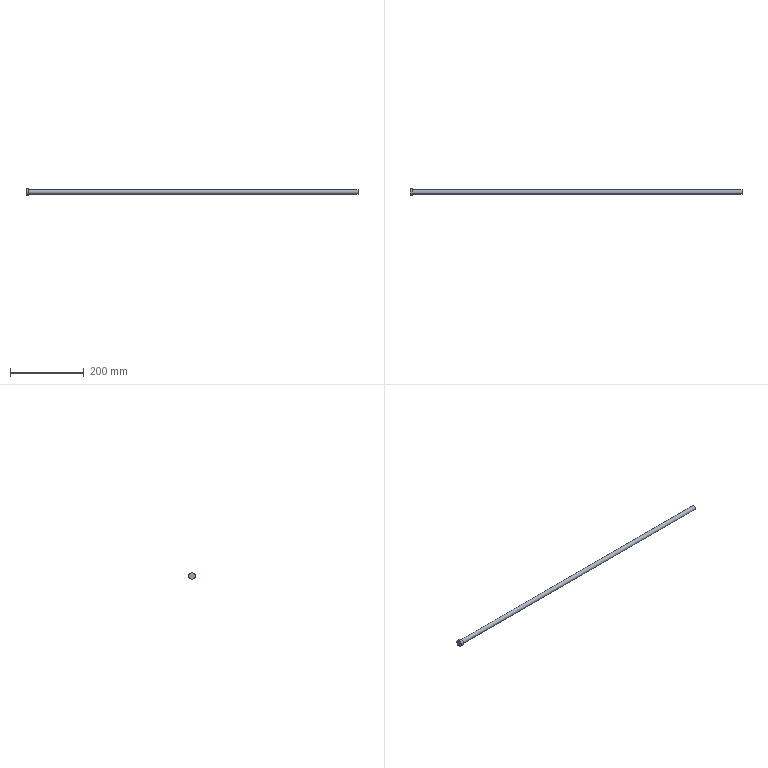Part | STEP file | solid 39 | 1 solid | 5 faces | box 901 x 18 x 18 mm | volume 103032 mm3 | plane 3 | cylinder 2 | commonest cylinder face diameters 12 x1 18 x1